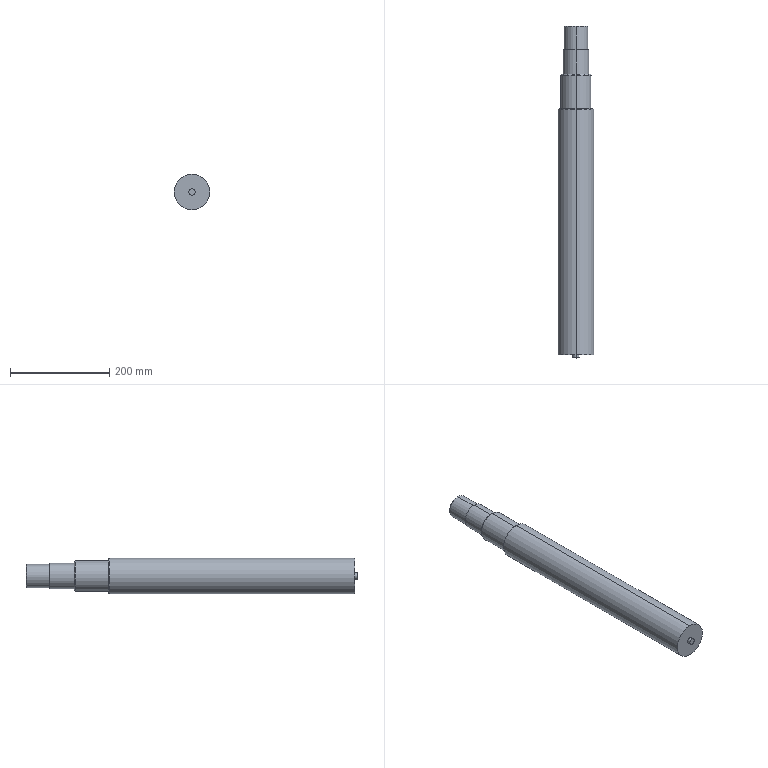Part | STEP file | 2. Piston Rod | 1 solid | 22 faces | box 71.582 x 670.101 x 71.582 mm | volume 2394238 mm3 | cylinder 10 | cone 6 | plane 6 | commonest cylinder face diameters 12.525 x2 47.345 x2 51.704 x2 61.374 x2 71.582 x2
STEP:
#1=CARTESIAN_POINT('',(0.,0.,35.791));
#2=VERTEX_POINT('',#1);
#3=CARTESIAN_POINT('',(0.,0.,-35.791));
#4=VERTEX_POINT('',#3);
#5=CARTESIAN_POINT('',(0.,0.,0.));
#6=DIRECTION('',(0.,1.,0.));
#7=DIRECTION('',(0.,0.,1.));
#8=AXIS2_PLACEMENT_3D('',#5,#6,#7);
#9=CIRCLE('',#8,35.791);
#10=EDGE_CURVE('',#2,#4,#9,.T.);
#11=ORIENTED_EDGE('',*,*,#10,.T.);
#12=CARTESIAN_POINT('',(0.,496.,-35.791));
#13=VERTEX_POINT('',#12);
#14=CARTESIAN_POINT('',(0.,-6.263,-35.791));
#15=DIRECTION('',(0.,1.,0.));
#16=VECTOR('',#15,1000.);
#17=LINE('',#14,#16);
#18=EDGE_CURVE('',#4,#13,#17,.T.);
#19=ORIENTED_EDGE('',*,*,#18,.T.);
#20=CARTESIAN_POINT('',(0.,496.,35.791));
#21=VERTEX_POINT('',#20);
#22=CARTESIAN_POINT('',(0.,496.,0.));
#23=DIRECTION('',(0.,1.,0.));
#24=DIRECTION('',(0.,0.,1.));
#25=AXIS2_PLACEMENT_3D('',#22,#23,#24);
#26=CIRCLE('',#25,35.791);
#27=EDGE_CURVE('',#21,#13,#26,.T.);
#28=ORIENTED_EDGE('',*,*,#27,.F.);
#29=CARTESIAN_POINT('',(0.,-6.263,35.791));
#30=DIRECTION('',(0.,1.,0.));
#31=VECTOR('',#30,1000.);
#32=LINE('',#29,#31);
#33=EDGE_CURVE('',#2,#21,#32,.T.);
#34=ORIENTED_EDGE('',*,*,#33,.F.);
#35=EDGE_LOOP('',(#11,#19,#28,#34));
#36=FACE_OUTER_BOUND('',#35,.T.);
#37=CARTESIAN_POINT('',(0.,-6.263,0.));
#38=DIRECTION('',(0.,1.,0.));
#39=DIRECTION('',(0.,0.,1.));
#40=AXIS2_PLACEMENT_3D('',#37,#38,#39);
#41=CYLINDRICAL_SURFACE('',#40,35.791);
#42=ADVANCED_FACE('',(#36),#41,.T.);
#43=CARTESIAN_POINT('',(0.,497.253,34.538));
#44=VERTEX_POINT('',#43);
#45=CARTESIAN_POINT('',(0.,497.253,-34.538));
#46=VERTEX_POINT('',#45);
#47=CARTESIAN_POINT('',(0.,497.253,0.));
#48=DIRECTION('',(0.,1.,0.));
#49=DIRECTION('',(0.,0.,1.));
#50=AXIS2_PLACEMENT_3D('',#47,#48,#49);
#51=CIRCLE('',#50,34.538);
#52=EDGE_CURVE('',#44,#46,#51,.T.);
#53=ORIENTED_EDGE('',*,*,#52,.F.);
#54=CARTESIAN_POINT('',(0.,497.253,34.538));
#55=DIRECTION('',(0.,-0.7071,0.7071));
#56=VECTOR('',#55,1000.);
#57=LINE('',#54,#56);
#58=EDGE_CURVE('',#44,#21,#57,.T.);
#59=ORIENTED_EDGE('',*,*,#58,.T.);
#60=ORIENTED_EDGE('',*,*,#27,.T.);
#61=CARTESIAN_POINT('',(0.,497.253,-34.538));
#62=DIRECTION('',(0.,-0.7071,-0.7071));
#63=VECTOR('',#62,1000.);
#64=LINE('',#61,#63);
#65=EDGE_CURVE('',#46,#13,#64,.T.);
#66=ORIENTED_EDGE('',*,*,#65,.F.);
#67=EDGE_LOOP('',(#53,#59,#60,#66));
#68=FACE_OUTER_BOUND('',#67,.T.);
#69=CARTESIAN_POINT('',(0.,497.253,0.));
#70=DIRECTION('',(0.,-1.,0.));
#71=DIRECTION('',(0.,0.,-1.));
#72=AXIS2_PLACEMENT_3D('',#69,#70,#71);
#73=CONICAL_SURFACE('',#72,34.538,0.7854);
#74=ADVANCED_FACE('',(#68),#73,.T.);
#75=CARTESIAN_POINT('',(0.,497.253,30.687));
#76=VERTEX_POINT('',#75);
#77=CARTESIAN_POINT('',(0.,497.253,-30.687));
#78=VERTEX_POINT('',#77);
#79=CARTESIAN_POINT('',(0.,497.253,0.));
#80=DIRECTION('',(0.,1.,0.));
#81=DIRECTION('',(0.,0.,1.));
#82=AXIS2_PLACEMENT_3D('',#79,#80,#81);
#83=CIRCLE('',#82,30.687);
#84=EDGE_CURVE('',#76,#78,#83,.T.);
#85=ORIENTED_EDGE('',*,*,#84,.T.);
#86=CARTESIAN_POINT('',(0.,564.889,-30.687));
#87=VERTEX_POINT('',#86);
#88=CARTESIAN_POINT('',(0.,-6.263,-30.687));
#89=DIRECTION('',(0.,1.,0.));
#90=VECTOR('',#89,1000.);
#91=LINE('',#88,#90);
#92=EDGE_CURVE('',#78,#87,#91,.T.);
#93=ORIENTED_EDGE('',*,*,#92,.T.);
#94=CARTESIAN_POINT('',(0.,564.889,30.687));
#95=VERTEX_POINT('',#94);
#96=CARTESIAN_POINT('',(0.,564.889,0.));
#97=DIRECTION('',(0.,1.,0.));
#98=DIRECTION('',(0.,0.,1.));
#99=AXIS2_PLACEMENT_3D('',#96,#97,#98);
#100=CIRCLE('',#99,30.687);
#101=EDGE_CURVE('',#95,#87,#100,.T.);
#102=ORIENTED_EDGE('',*,*,#101,.F.);
#103=CARTESIAN_POINT('',(0.,-6.263,30.687));
#104=DIRECTION('',(0.,1.,0.));
#105=VECTOR('',#104,1000.);
#106=LINE('',#103,#105);
#107=EDGE_CURVE('',#76,#95,#106,.T.);
#108=ORIENTED_EDGE('',*,*,#107,.F.);
#109=EDGE_LOOP('',(#85,#93,#102,#108));
#110=FACE_OUTER_BOUND('',#109,.T.);
#111=CARTESIAN_POINT('',(0.,-6.263,0.));
#112=DIRECTION('',(0.,1.,0.));
#113=DIRECTION('',(0.,0.,1.));
#114=AXIS2_PLACEMENT_3D('',#111,#112,#113);
#115=CYLINDRICAL_SURFACE('',#114,30.687);
#116=ADVANCED_FACE('',(#110),#115,.T.);
#117=CARTESIAN_POINT('',(0.,566.141,29.434));
#118=VERTEX_POINT('',#117);
#119=CARTESIAN_POINT('',(0.,566.141,-29.434));
#120=VERTEX_POINT('',#119);
#121=CARTESIAN_POINT('',(0.,566.141,0.));
#122=DIRECTION('',(0.,1.,0.));
#123=DIRECTION('',(0.,0.,1.));
#124=AXIS2_PLACEMENT_3D('',#121,#122,#123);
#125=CIRCLE('',#124,29.434);
#126=EDGE_CURVE('',#118,#120,#125,.T.);
#127=ORIENTED_EDGE('',*,*,#126,.F.);
#128=CARTESIAN_POINT('',(0.,566.141,29.434));
#129=DIRECTION('',(0.,-0.7071,0.7071));
#130=VECTOR('',#129,1000.);
#131=LINE('',#128,#130);
#132=EDGE_CURVE('',#118,#95,#131,.T.);
#133=ORIENTED_EDGE('',*,*,#132,.T.);
#134=ORIENTED_EDGE('',*,*,#101,.T.);
#135=CARTESIAN_POINT('',(0.,566.141,-29.434));
#136=DIRECTION('',(0.,-0.7071,-0.7071));
#137=VECTOR('',#136,1000.);
#138=LINE('',#135,#137);
#139=EDGE_CURVE('',#120,#87,#138,.T.);
#140=ORIENTED_EDGE('',*,*,#139,.F.);
#141=EDGE_LOOP('',(#127,#133,#134,#140));
#142=FACE_OUTER_BOUND('',#141,.T.);
#143=CARTESIAN_POINT('',(0.,566.141,0.));
#144=DIRECTION('',(0.,-1.,0.));
#145=DIRECTION('',(0.,0.,-1.));
#146=AXIS2_PLACEMENT_3D('',#143,#144,#145);
#147=CONICAL_SURFACE('',#146,29.434,0.7854);
#148=ADVANCED_FACE('',(#142),#147,.T.);
#149=CARTESIAN_POINT('',(0.,566.141,25.852));
#150=VERTEX_POINT('',#149);
#151=CARTESIAN_POINT('',(0.,566.141,-25.852));
#152=VERTEX_POINT('',#151);
#153=CARTESIAN_POINT('',(0.,566.141,0.));
#154=DIRECTION('',(0.,1.,0.));
#155=DIRECTION('',(0.,0.,1.));
#156=AXIS2_PLACEMENT_3D('',#153,#154,#155);
#157=CIRCLE('',#156,25.852);
#158=EDGE_CURVE('',#150,#152,#157,.T.);
#159=ORIENTED_EDGE('',*,*,#158,.T.);
#160=CARTESIAN_POINT('',(0.,616.242,-25.852));
#161=VERTEX_POINT('',#160);
#162=CARTESIAN_POINT('',(0.,-6.263,-25.852));
#163=DIRECTION('',(0.,1.,0.));
#164=VECTOR('',#163,1000.);
#165=LINE('',#162,#164);
#166=EDGE_CURVE('',#152,#161,#165,.T.);
#167=ORIENTED_EDGE('',*,*,#166,.T.);
#168=CARTESIAN_POINT('',(0.,616.242,25.852));
#169=VERTEX_POINT('',#168);
#170=CARTESIAN_POINT('',(0.,616.242,0.));
#171=DIRECTION('',(0.,1.,0.));
#172=DIRECTION('',(0.,0.,1.));
#173=AXIS2_PLACEMENT_3D('',#170,#171,#172);
#174=CIRCLE('',#173,25.852);
#175=EDGE_CURVE('',#169,#161,#174,.T.);
#176=ORIENTED_EDGE('',*,*,#175,.F.);
#177=CARTESIAN_POINT('',(0.,-6.263,25.852));
#178=DIRECTION('',(0.,1.,0.));
#179=VECTOR('',#178,1000.);
#180=LINE('',#177,#179);
#181=EDGE_CURVE('',#150,#169,#180,.T.);
#182=ORIENTED_EDGE('',*,*,#181,.F.);
#183=EDGE_LOOP('',(#159,#167,#176,#182));
#184=FACE_OUTER_BOUND('',#183,.T.);
#185=CARTESIAN_POINT('',(0.,-6.263,0.));
#186=DIRECTION('',(0.,1.,0.));
#187=DIRECTION('',(0.,0.,1.));
#188=AXIS2_PLACEMENT_3D('',#185,#186,#187);
#189=CYLINDRICAL_SURFACE('',#188,25.852);
#190=ADVANCED_FACE('',(#184),#189,.T.);
#191=CARTESIAN_POINT('',(0.,616.242,23.673));
#192=VERTEX_POINT('',#191);
#193=CARTESIAN_POINT('',(0.,616.242,-23.673));
#194=VERTEX_POINT('',#193);
#195=CARTESIAN_POINT('',(0.,616.242,0.));
#196=DIRECTION('',(0.,1.,0.));
#197=DIRECTION('',(0.,0.,1.));
#198=AXIS2_PLACEMENT_3D('',#195,#196,#197);
#199=CIRCLE('',#198,23.673);
#200=EDGE_CURVE('',#192,#194,#199,.T.);
#201=ORIENTED_EDGE('',*,*,#200,.T.);
#202=CARTESIAN_POINT('',(0.,662.586,-23.673));
#203=VERTEX_POINT('',#202);
#204=CARTESIAN_POINT('',(0.,-6.263,-23.673));
#205=DIRECTION('',(0.,1.,0.));
#206=VECTOR('',#205,1000.);
#207=LINE('',#204,#206);
#208=EDGE_CURVE('',#194,#203,#207,.T.);
#209=ORIENTED_EDGE('',*,*,#208,.T.);
#210=CARTESIAN_POINT('',(0.,662.586,23.673));
#211=VERTEX_POINT('',#210);
#212=CARTESIAN_POINT('',(0.,662.586,0.));
#213=DIRECTION('',(0.,1.,0.));
#214=DIRECTION('',(0.,0.,1.));
#215=AXIS2_PLACEMENT_3D('',#212,#213,#214);
#216=CIRCLE('',#215,23.673);
#217=EDGE_CURVE('',#211,#203,#216,.T.);
#218=ORIENTED_EDGE('',*,*,#217,.F.);
#219=CARTESIAN_POINT('',(0.,-6.263,23.673));
#220=DIRECTION('',(0.,1.,0.));
#221=VECTOR('',#220,1000.);
#222=LINE('',#219,#221);
#223=EDGE_CURVE('',#192,#211,#222,.T.);
#224=ORIENTED_EDGE('',*,*,#223,.F.);
#225=EDGE_LOOP('',(#201,#209,#218,#224));
#226=FACE_OUTER_BOUND('',#225,.T.);
#227=CARTESIAN_POINT('',(0.,-6.263,0.));
#228=DIRECTION('',(0.,1.,0.));
#229=DIRECTION('',(0.,0.,1.));
#230=AXIS2_PLACEMENT_3D('',#227,#228,#229);
#231=CYLINDRICAL_SURFACE('',#230,23.673);
#232=ADVANCED_FACE('',(#226),#231,.T.);
#233=CARTESIAN_POINT('',(0.,663.838,22.42));
#234=VERTEX_POINT('',#233);
#235=CARTESIAN_POINT('',(0.,663.838,-22.42));
#236=VERTEX_POINT('',#235);
#237=CARTESIAN_POINT('',(0.,663.838,0.));
#238=DIRECTION('',(0.,1.,0.));
#239=DIRECTION('',(0.,0.,1.));
#240=AXIS2_PLACEMENT_3D('',#237,#238,#239);
#241=CIRCLE('',#240,22.42);
#242=EDGE_CURVE('',#234,#236,#241,.T.);
#243=ORIENTED_EDGE('',*,*,#242,.F.);
#244=CARTESIAN_POINT('',(0.,663.838,22.42));
#245=DIRECTION('',(0.,-0.7071,0.7071));
#246=VECTOR('',#245,1000.);
#247=LINE('',#244,#246);
#248=EDGE_CURVE('',#234,#211,#247,.T.);
#249=ORIENTED_EDGE('',*,*,#248,.T.);
#250=ORIENTED_EDGE('',*,*,#217,.T.);
#251=CARTESIAN_POINT('',(0.,663.838,-22.42));
#252=DIRECTION('',(0.,-0.7071,-0.7071));
#253=VECTOR('',#252,1000.);
#254=LINE('',#251,#253);
#255=EDGE_CURVE('',#236,#203,#254,.T.);
#256=ORIENTED_EDGE('',*,*,#255,.F.);
#257=EDGE_LOOP('',(#243,#249,#250,#256));
#258=FACE_OUTER_BOUND('',#257,.T.);
#259=CARTESIAN_POINT('',(0.,663.838,0.));
#260=DIRECTION('',(0.,-1.,0.));
#261=DIRECTION('',(0.,0.,-1.));
#262=AXIS2_PLACEMENT_3D('',#259,#260,#261);
#263=CONICAL_SURFACE('',#262,22.42,0.7854);
#264=ADVANCED_FACE('',(#258),#263,.T.);
#265=CARTESIAN_POINT('',(0.,-6.263,6.263));
#266=VERTEX_POINT('',#265);
#267=CARTESIAN_POINT('',(0.,-6.263,-6.263));
#268=VERTEX_POINT('',#267);
#269=CARTESIAN_POINT('',(0.,-6.263,0.));
#270=DIRECTION('',(0.,1.,0.));
#271=DIRECTION('',(0.,0.,1.));
#272=AXIS2_PLACEMENT_3D('',#269,#270,#271);
#273=CIRCLE('',#272,6.263);
#274=EDGE_CURVE('',#266,#268,#273,.T.);
#275=ORIENTED_EDGE('',*,*,#274,.T.);
#276=CARTESIAN_POINT('',(0.,0.,-6.263));
#277=VERTEX_POINT('',#276);
#278=CARTESIAN_POINT('',(0.,-6.263,-6.263));
#279=DIRECTION('',(0.,1.,0.));
#280=VECTOR('',#279,1000.);
#281=LINE('',#278,#280);
#282=EDGE_CURVE('',#268,#277,#281,.T.);
#283=ORIENTED_EDGE('',*,*,#282,.T.);
#284=CARTESIAN_POINT('',(0.,0.,6.263));
#285=VERTEX_POINT('',#284);
#286=CARTESIAN_POINT('',(0.,0.,0.));
#287=DIRECTION('',(0.,1.,0.));
#288=DIRECTION('',(0.,0.,1.));
#289=AXIS2_PLACEMENT_3D('',#286,#287,#288);
#290=CIRCLE('',#289,6.263);
#291=EDGE_CURVE('',#285,#277,#290,.T.);
#292=ORIENTED_EDGE('',*,*,#291,.F.);
#293=CARTESIAN_POINT('',(0.,-6.263,6.263));
#294=DIRECTION('',(0.,1.,0.));
#295=VECTOR('',#294,1000.);
#296=LINE('',#293,#295);
#297=EDGE_CURVE('',#266,#285,#296,.T.);
#298=ORIENTED_EDGE('',*,*,#297,.F.);
#299=EDGE_LOOP('',(#275,#283,#292,#298));
#300=FACE_OUTER_BOUND('',#299,.T.);
#301=CARTESIAN_POINT('',(0.,-6.263,0.));
#302=DIRECTION('',(0.,1.,0.));
#303=DIRECTION('',(0.,0.,1.));
#304=AXIS2_PLACEMENT_3D('',#301,#302,#303);
#305=CYLINDRICAL_SURFACE('',#304,6.263);
#306=ADVANCED_FACE('',(#300),#305,.T.);
#307=ORIENTED_EDGE('',*,*,#282,.F.);
#308=CARTESIAN_POINT('',(0.,-6.263,0.));
#309=DIRECTION('',(0.,1.,0.));
#310=DIRECTION('',(0.,0.,1.));
#311=AXIS2_PLACEMENT_3D('',#308,#309,#310);
#312=CIRCLE('',#311,6.263);
#313=EDGE_CURVE('',#268,#266,#312,.T.);
#314=ORIENTED_EDGE('',*,*,#313,.T.);
#315=ORIENTED_EDGE('',*,*,#297,.T.);
#316=CARTESIAN_POINT('',(0.,0.,0.));
#317=DIRECTION('',(0.,1.,0.));
#318=DIRECTION('',(0.,0.,1.));
#319=AXIS2_PLACEMENT_3D('',#316,#317,#318);
#320=CIRCLE('',#319,6.263);
#321=EDGE_CURVE('',#277,#285,#320,.T.);
#322=ORIENTED_EDGE('',*,*,#321,.F.);
#323=EDGE_LOOP('',(#307,#314,#315,#322));
#324=FACE_OUTER_BOUND('',#323,.T.);
#325=CARTESIAN_POINT('',(0.,-6.263,0.));
#326=DIRECTION('',(0.,1.,0.));
#327=DIRECTION('',(0.,0.,1.));
#328=AXIS2_PLACEMENT_3D('',#325,#326,#327);
#329=CYLINDRICAL_SURFACE('',#328,6.263);
#330=ADVANCED_FACE('',(#324),#329,.T.);
#331=ORIENTED_EDGE('',*,*,#274,.F.);
#332=ORIENTED_EDGE('',*,*,#313,.F.);
#333=EDGE_LOOP('',(#331,#332));
#334=FACE_OUTER_BOUND('',#333,.T.);
#335=CARTESIAN_POINT('',(6.263,-6.263,0.));
#336=DIRECTION('',(0.,-1.,0.));
#337=DIRECTION('',(0.,0.,-1.));
#338=AXIS2_PLACEMENT_3D('',#335,#336,#337);
#339=PLANE('',#338);
#340=ADVANCED_FACE('',(#334),#339,.T.);
#341=CARTESIAN_POINT('',(0.,663.838,0.));
#342=DIRECTION('',(0.,1.,0.));
#343=DIRECTION('',(0.,0.,1.));
#344=AXIS2_PLACEMENT_3D('',#341,#342,#343);
#345=CIRCLE('',#344,22.42);
#346=EDGE_CURVE('',#236,#234,#345,.T.);
#347=ORIENTED_EDGE('',*,*,#346,.T.);
#348=ORIENTED_EDGE('',*,*,#242,.T.);
#349=EDGE_LOOP('',(#347,#348));
#350=FACE_OUTER_BOUND('',#349,.T.);
#351=CARTESIAN_POINT('',(0.,663.838,0.));
#352=DIRECTION('',(0.,1.,0.));
#353=DIRECTION('',(0.,0.,1.));
#354=AXIS2_PLACEMENT_3D('',#351,#352,#353);
#355=PLANE('',#354);
#356=ADVANCED_FACE('',(#350),#355,.T.);
#357=ORIENTED_EDGE('',*,*,#248,.F.);
#358=ORIENTED_EDGE('',*,*,#346,.F.);
#359=ORIENTED_EDGE('',*,*,#255,.T.);
#360=CARTESIAN_POINT('',(0.,662.586,0.));
#361=DIRECTION('',(0.,1.,0.));
#362=DIRECTION('',(0.,0.,1.));
#363=AXIS2_PLACEMENT_3D('',#360,#361,#362);
#364=CIRCLE('',#363,23.673);
#365=EDGE_CURVE('',#203,#211,#364,.T.);
#366=ORIENTED_EDGE('',*,*,#365,.T.);
#367=EDGE_LOOP('',(#357,#358,#359,#366));
#368=FACE_OUTER_BOUND('',#367,.T.);
#369=CARTESIAN_POINT('',(0.,663.838,0.));
#370=DIRECTION('',(0.,-1.,0.));
#371=DIRECTION('',(0.,0.,-1.));
#372=AXIS2_PLACEMENT_3D('',#369,#370,#371);
#373=CONICAL_SURFACE('',#372,22.42,0.7854);
#374=ADVANCED_FACE('',(#368),#373,.T.);
#375=ORIENTED_EDGE('',*,*,#208,.F.);
#376=CARTESIAN_POINT('',(0.,616.242,0.));
#377=DIRECTION('',(0.,1.,0.));
#378=DIRECTION('',(0.,0.,1.));
#379=AXIS2_PLACEMENT_3D('',#376,#377,#378);
#380=CIRCLE('',#379,23.673);
#381=EDGE_CURVE('',#194,#192,#380,.T.);
#382=ORIENTED_EDGE('',*,*,#381,.T.);
#383=ORIENTED_EDGE('',*,*,#223,.T.);
#384=ORIENTED_EDGE('',*,*,#365,.F.);
#385=EDGE_LOOP('',(#375,#382,#383,#384));
#386=FACE_OUTER_BOUND('',#385,.T.);
#387=CARTESIAN_POINT('',(0.,-6.263,0.));
#388=DIRECTION('',(0.,1.,0.));
#389=DIRECTION('',(0.,0.,1.));
#390=AXIS2_PLACEMENT_3D('',#387,#388,#389);
#391=CYLINDRICAL_SURFACE('',#390,23.673);
#392=ADVANCED_FACE('',(#386),#391,.T.);
#393=ORIENTED_EDGE('',*,*,#175,.T.);
#394=CARTESIAN_POINT('',(0.,616.242,0.));
#395=DIRECTION('',(0.,1.,0.));
#396=DIRECTION('',(0.,0.,1.));
#397=AXIS2_PLACEMENT_3D('',#394,#395,#396);
#398=CIRCLE('',#397,25.852);
#399=EDGE_CURVE('',#161,#169,#398,.T.);
#400=ORIENTED_EDGE('',*,*,#399,.T.);
#401=EDGE_LOOP('',(#393,#400));
#402=FACE_OUTER_BOUND('',#401,.T.);
#403=ORIENTED_EDGE('',*,*,#200,.F.);
#404=ORIENTED_EDGE('',*,*,#381,.F.);
#405=EDGE_LOOP('',(#403,#404));
#406=FACE_BOUND('',#405,.T.);
#407=CARTESIAN_POINT('',(23.673,616.242,0.));
#408=DIRECTION('',(0.,1.,0.));
#409=DIRECTION('',(0.,0.,1.));
#410=AXIS2_PLACEMENT_3D('',#407,#408,#409);
#411=PLANE('',#410);
#412=ADVANCED_FACE('',(#402,#406),#411,.T.);
#413=ORIENTED_EDGE('',*,*,#166,.F.);
#414=CARTESIAN_POINT('',(0.,566.141,0.));
#415=DIRECTION('',(0.,1.,0.));
#416=DIRECTION('',(0.,0.,1.));
#417=AXIS2_PLACEMENT_3D('',#414,#415,#416);
#418=CIRCLE('',#417,25.852);
#419=EDGE_CURVE('',#152,#150,#418,.T.);
#420=ORIENTED_EDGE('',*,*,#419,.T.);
#421=ORIENTED_EDGE('',*,*,#181,.T.);
#422=ORIENTED_EDGE('',*,*,#399,.F.);
#423=EDGE_LOOP('',(#413,#420,#421,#422));
#424=FACE_OUTER_BOUND('',#423,.T.);
#425=CARTESIAN_POINT('',(0.,-6.263,0.));
#426=DIRECTION('',(0.,1.,0.));
#427=DIRECTION('',(0.,0.,1.));
#428=AXIS2_PLACEMENT_3D('',#425,#426,#427);
#429=CYLINDRICAL_SURFACE('',#428,25.852);
#430=ADVANCED_FACE('',(#424),#429,.T.);
#431=CARTESIAN_POINT('',(0.,566.141,0.));
#432=DIRECTION('',(0.,1.,0.));
#433=DIRECTION('',(0.,0.,1.));
#434=AXIS2_PLACEMENT_3D('',#431,#432,#433);
#435=CIRCLE('',#434,29.434);
#436=EDGE_CURVE('',#120,#118,#435,.T.);
#437=ORIENTED_EDGE('',*,*,#436,.T.);
#438=ORIENTED_EDGE('',*,*,#126,.T.);
#439=EDGE_LOOP('',(#437,#438));
#440=FACE_OUTER_BOUND('',#439,.T.);
#441=ORIENTED_EDGE('',*,*,#158,.F.);
#442=ORIENTED_EDGE('',*,*,#419,.F.);
#443=EDGE_LOOP('',(#441,#442));
#444=FACE_BOUND('',#443,.T.);
#445=CARTESIAN_POINT('',(25.852,566.141,0.));
#446=DIRECTION('',(0.,1.,0.));
#447=DIRECTION('',(0.,0.,1.));
#448=AXIS2_PLACEMENT_3D('',#445,#446,#447);
#449=PLANE('',#448);
#450=ADVANCED_FACE('',(#440,#444),#449,.T.);
#451=ORIENTED_EDGE('',*,*,#132,.F.);
#452=ORIENTED_EDGE('',*,*,#436,.F.);
#453=ORIENTED_EDGE('',*,*,#139,.T.);
#454=CARTESIAN_POINT('',(0.,564.889,0.));
#455=DIRECTION('',(0.,1.,0.));
#456=DIRECTION('',(0.,0.,1.));
#457=AXIS2_PLACEMENT_3D('',#454,#455,#456);
#458=CIRCLE('',#457,30.687);
#459=EDGE_CURVE('',#87,#95,#458,.T.);
#460=ORIENTED_EDGE('',*,*,#459,.T.);
#461=EDGE_LOOP('',(#451,#452,#453,#460));
#462=FACE_OUTER_BOUND('',#461,.T.);
#463=CARTESIAN_POINT('',(0.,566.141,0.));
#464=DIRECTION('',(0.,-1.,0.));
#465=DIRECTION('',(0.,0.,-1.));
#466=AXIS2_PLACEMENT_3D('',#463,#464,#465);
#467=CONICAL_SURFACE('',#466,29.434,0.7854);
#468=ADVANCED_FACE('',(#462),#467,.T.);
#469=ORIENTED_EDGE('',*,*,#92,.F.);
#470=CARTESIAN_POINT('',(0.,497.253,0.));
#471=DIRECTION('',(0.,1.,0.));
#472=DIRECTION('',(0.,0.,1.));
#473=AXIS2_PLACEMENT_3D('',#470,#471,#472);
#474=CIRCLE('',#473,30.687);
#475=EDGE_CURVE('',#78,#76,#474,.T.);
#476=ORIENTED_EDGE('',*,*,#475,.T.);
#477=ORIENTED_EDGE('',*,*,#107,.T.);
#478=ORIENTED_EDGE('',*,*,#459,.F.);
#479=EDGE_LOOP('',(#469,#476,#477,#478));
#480=FACE_OUTER_BOUND('',#479,.T.);
#481=CARTESIAN_POINT('',(0.,-6.263,0.));
#482=DIRECTION('',(0.,1.,0.));
#483=DIRECTION('',(0.,0.,1.));
#484=AXIS2_PLACEMENT_3D('',#481,#482,#483);
#485=CYLINDRICAL_SURFACE('',#484,30.687);
#486=ADVANCED_FACE('',(#480),#485,.T.);
#487=CARTESIAN_POINT('',(0.,497.253,0.));
#488=DIRECTION('',(0.,1.,0.));
#489=DIRECTION('',(0.,0.,1.));
#490=AXIS2_PLACEMENT_3D('',#487,#488,#489);
#491=CIRCLE('',#490,34.538);
#492=EDGE_CURVE('',#46,#44,#491,.T.);
#493=ORIENTED_EDGE('',*,*,#492,.T.);
#494=ORIENTED_EDGE('',*,*,#52,.T.);
#495=EDGE_LOOP('',(#493,#494));
#496=FACE_OUTER_BOUND('',#495,.T.);
#497=ORIENTED_EDGE('',*,*,#84,.F.);
#498=ORIENTED_EDGE('',*,*,#475,.F.);
#499=EDGE_LOOP('',(#497,#498));
#500=FACE_BOUND('',#499,.T.);
#501=CARTESIAN_POINT('',(30.687,497.253,0.));
#502=DIRECTION('',(0.,1.,0.));
#503=DIRECTION('',(0.,0.,1.));
#504=AXIS2_PLACEMENT_3D('',#501,#502,#503);
#505=PLANE('',#504);
#506=ADVANCED_FACE('',(#496,#500),#505,.T.);
#507=ORIENTED_EDGE('',*,*,#58,.F.);
#508=ORIENTED_EDGE('',*,*,#492,.F.);
#509=ORIENTED_EDGE('',*,*,#65,.T.);
#510=CARTESIAN_POINT('',(0.,496.,0.));
#511=DIRECTION('',(0.,1.,0.));
#512=DIRECTION('',(0.,0.,1.));
#513=AXIS2_PLACEMENT_3D('',#510,#511,#512);
#514=CIRCLE('',#513,35.791);
#515=EDGE_CURVE('',#13,#21,#514,.T.);
#516=ORIENTED_EDGE('',*,*,#515,.T.);
#517=EDGE_LOOP('',(#507,#508,#509,#516));
#518=FACE_OUTER_BOUND('',#517,.T.);
#519=CARTESIAN_POINT('',(0.,497.253,0.));
#520=DIRECTION('',(0.,-1.,0.));
#521=DIRECTION('',(0.,0.,-1.));
#522=AXIS2_PLACEMENT_3D('',#519,#520,#521);
#523=CONICAL_SURFACE('',#522,34.538,0.7854);
#524=ADVANCED_FACE('',(#518),#523,.T.);
#525=ORIENTED_EDGE('',*,*,#18,.F.);
#526=CARTESIAN_POINT('',(0.,0.,0.));
#527=DIRECTION('',(0.,1.,0.));
#528=DIRECTION('',(0.,0.,1.));
#529=AXIS2_PLACEMENT_3D('',#526,#527,#528);
#530=CIRCLE('',#529,35.791);
#531=EDGE_CURVE('',#4,#2,#530,.T.);
#532=ORIENTED_EDGE('',*,*,#531,.T.);
#533=ORIENTED_EDGE('',*,*,#33,.T.);
#534=ORIENTED_EDGE('',*,*,#515,.F.);
#535=EDGE_LOOP('',(#525,#532,#533,#534));
#536=FACE_OUTER_BOUND('',#535,.T.);
#537=CARTESIAN_POINT('',(0.,-6.263,0.));
#538=DIRECTION('',(0.,1.,0.));
#539=DIRECTION('',(0.,0.,1.));
#540=AXIS2_PLACEMENT_3D('',#537,#538,#539);
#541=CYLINDRICAL_SURFACE('',#540,35.791);
#542=ADVANCED_FACE('',(#536),#541,.T.);
#543=ORIENTED_EDGE('',*,*,#291,.T.);
#544=ORIENTED_EDGE('',*,*,#321,.T.);
#545=EDGE_LOOP('',(#543,#544));
#546=FACE_BOUND('',#545,.T.);
#547=ORIENTED_EDGE('',*,*,#10,.F.);
#548=ORIENTED_EDGE('',*,*,#531,.F.);
#549=EDGE_LOOP('',(#547,#548));
#550=FACE_OUTER_BOUND('',#549,.T.);
#551=CARTESIAN_POINT('',(35.791,0.,0.));
#552=DIRECTION('',(0.,-1.,0.));
#553=DIRECTION('',(0.,0.,-1.));
#554=AXIS2_PLACEMENT_3D('',#551,#552,#553);
#555=PLANE('',#554);
#556=ADVANCED_FACE('',(#546,#550),#555,.T.);
#557=CLOSED_SHELL('',(#42,#74,#116,#148,#190,#232,#264,#306,#330,#340,#356,#374,#392,#412,#430,#450,#468,#486,#506,#524,#542,#556));
#558=MANIFOLD_SOLID_BREP('',#557);
#559=CARTESIAN_POINT('',(0.,0.,0.));
#560=DIRECTION('',(0.,0.,1.));
#561=DIRECTION('',(1.,0.,0.));
#562=AXIS2_PLACEMENT_3D('',#559,#560,#561);
#563=(LENGTH_UNIT()NAMED_UNIT(*)SI_UNIT(.MILLI.,.METRE.));
#564=UNCERTAINTY_MEASURE_WITH_UNIT(LENGTH_MEASURE(0.00001),#563,'','');
#565=(NAMED_UNIT(*)PLANE_ANGLE_UNIT()SI_UNIT($,.RADIAN.));
#566=(NAMED_UNIT(*)SI_UNIT($,.STERADIAN.)SOLID_ANGLE_UNIT());
#567=(GEOMETRIC_REPRESENTATION_CONTEXT(3)GLOBAL_UNCERTAINTY_ASSIGNED_CONTEXT((#564))GLOBAL_UNIT_ASSIGNED_CONTEXT((#563,#565,#566))REPRESENTATION_CONTEXT('',''));
#568=ADVANCED_BREP_SHAPE_REPRESENTATION('',(#558,#562),#567);